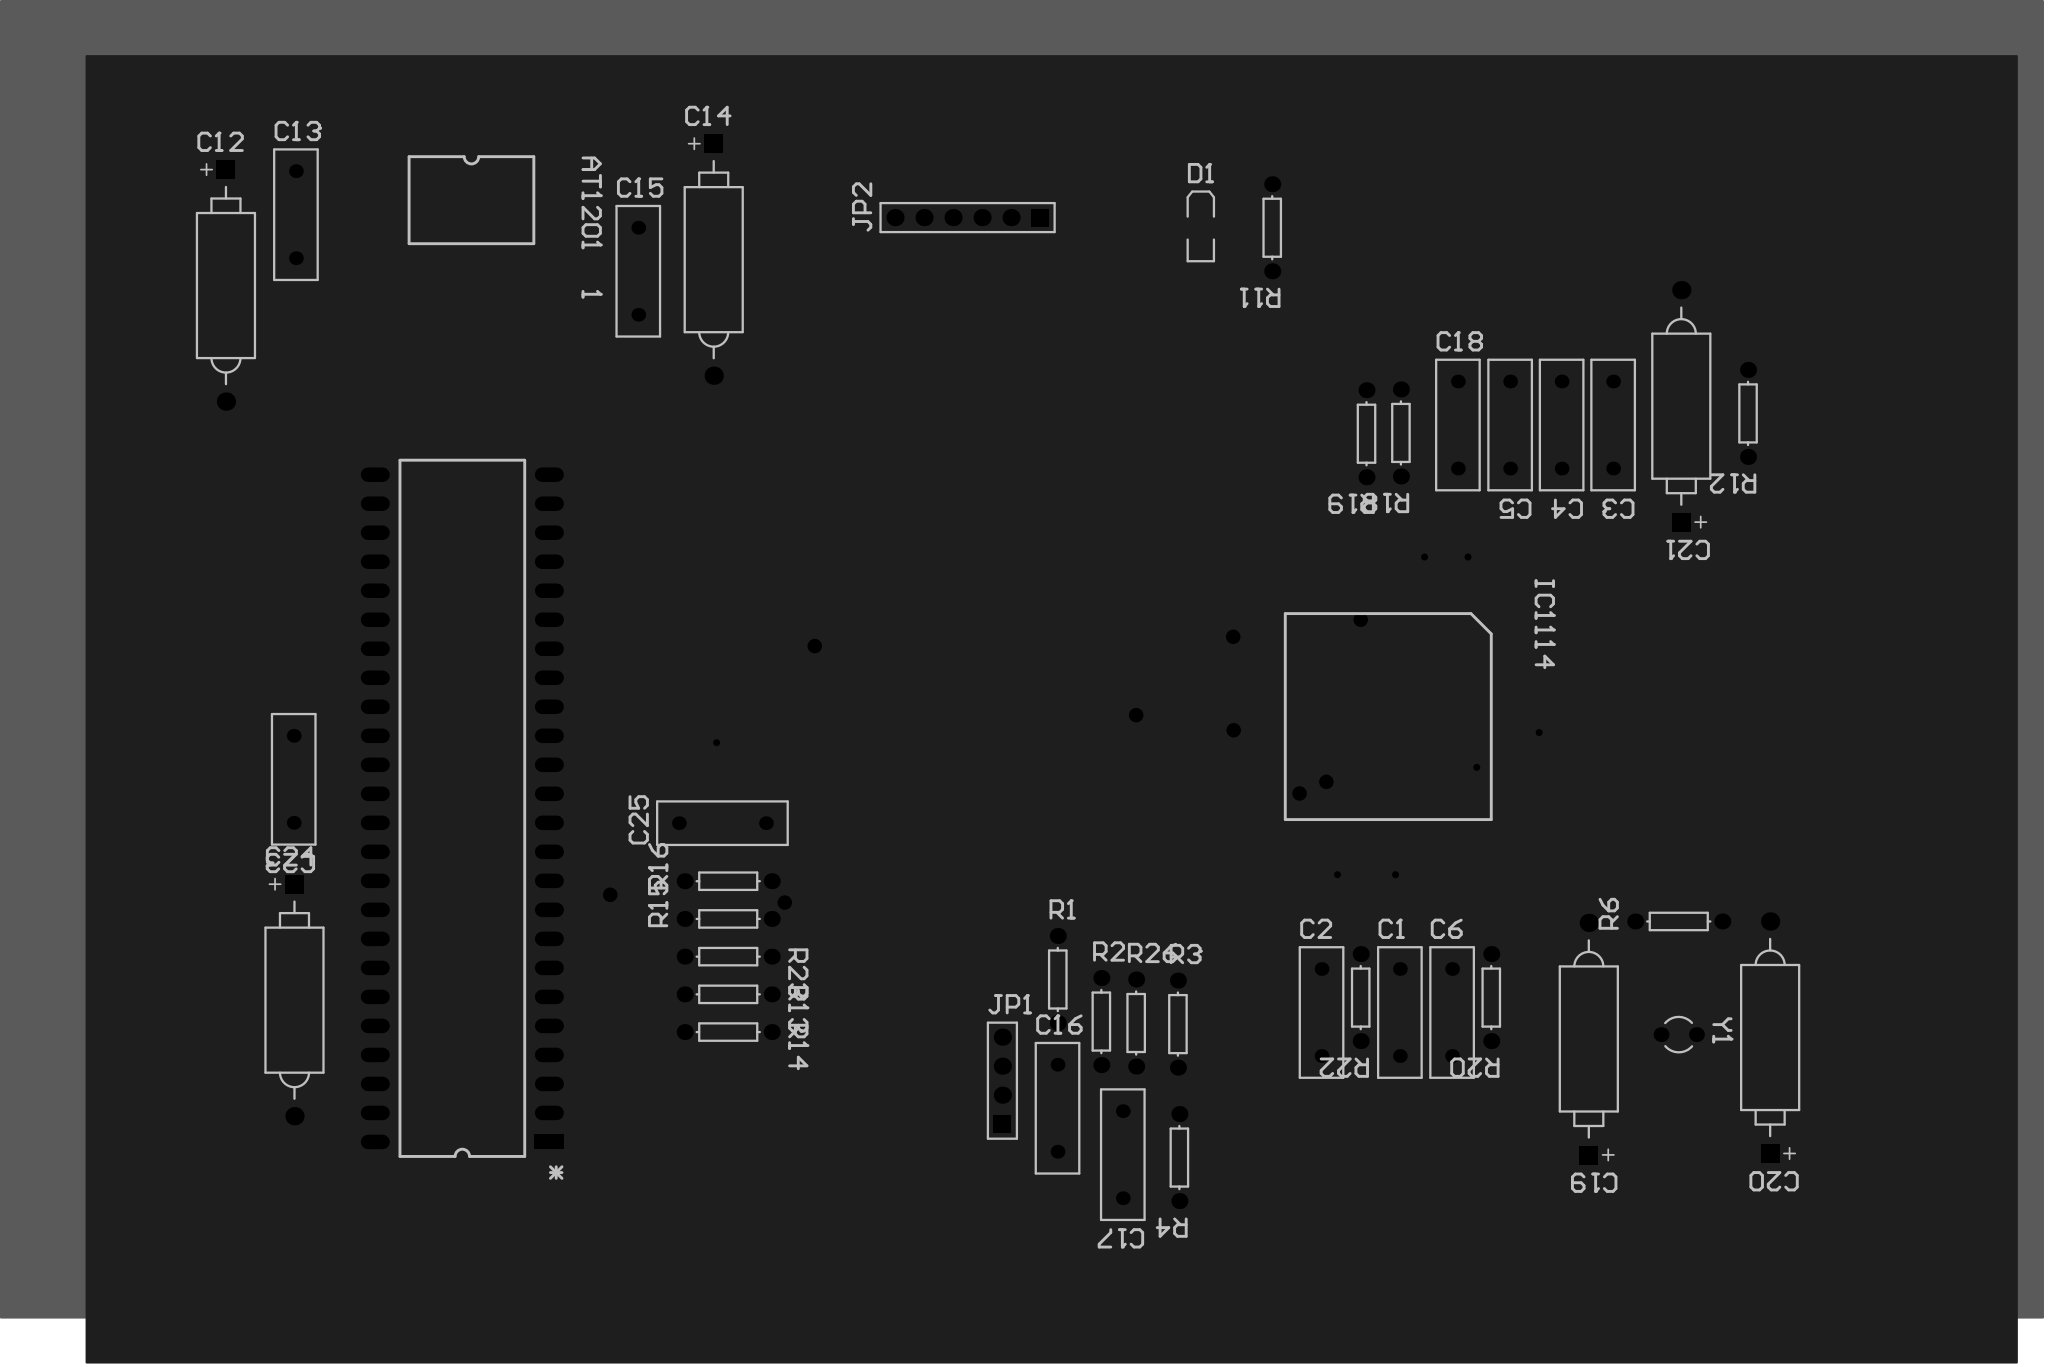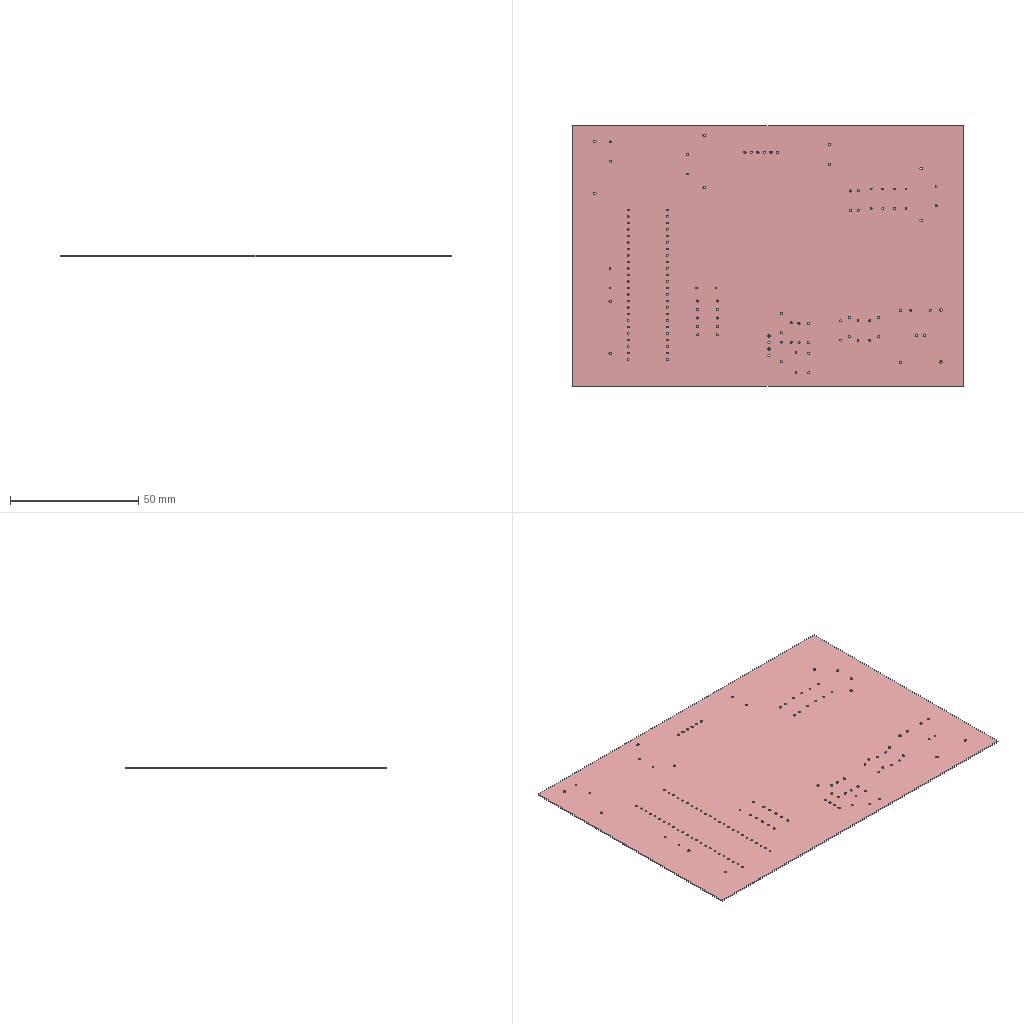Circuit board layout | Altium Designer | box 152.4 x 101.6 x 0.4 mm
Layer stack:
# Altium Designer layer stack of  (unit mm; dielectric type: 0 none, 1 core, 2 prepreg, 3 surface material)
index,name,kind,layer,copper_thickness_mm,dielectric_type,dielectric_thickness_mm,dielectric_material,dielectric_constant
0,Top Paste Mask Layer,other,,,,,,
1,Top Silkscreen Layer,other,,,,,,
2,Top Solder Mask Layer,dielectric,,,3,0.0102,Solder Resist,3.5
3,Top Layer,copper,Top Layer,0.0356,,,,
4,Dielectric 1,dielectric,,,3,0.32,FR-4,4.8
5,Bottom Layer,copper,Bottom Layer,0.0356,,,,
6,Bottom Solder Mask Layer,dielectric,,,3,0.0102,Solder Resist,3.5
7,Bottom Silkscreen Layer,other,,,,,,
8,Bottom Paste Mask Layer,other,,,,,,
# drill layer pairs: low layer,high layer
drill_pair,Top Layer,Bottom Layer
Part placement:
Designator,Comment,Layer,Footprint,Center-X(mm),Center-Y(mm),Rotation
Y1,,TopLayer,R38,223.17,104.998,270
R1,Res1,TopLayer,AXIAL-0.3,168.806,109.824,90
R26,,TopLayer,AXIAL-0.3,175.667,106.014,90
R23,,TopLayer,AXIAL-0.3,139.954,111.825,0
R22,,TopLayer,AXIAL-0.3,195.326,108.239,270
R20,,TopLayer,AXIAL-0.3,206.756,108.239,270
R19,,TopLayer,AXIAL-0.3,195.834,157.607,270
R18,,TopLayer,AXIAL-0.3,198.846,157.676,270
R16,,TopLayer,AXIAL-0.3,139.954,118.429,180
R15,,TopLayer,AXIAL-0.3,139.954,115.127,180
R14,,TopLayer,AXIAL-0.3,139.954,105.221,0
R13,,TopLayer,AXIAL-0.3,139.954,108.523,0
R12,,TopLayer,AXIAL-0.3,229.235,159.385,270
R11,,TopLayer,AXIAL-0.3,187.579,175.641,270
R6,,TopLayer,AXIAL-0.3,223.17,114.904,180
R4,,TopLayer,AXIAL-0.3,179.451,94.234,270
R3,,TopLayer,AXIAL-0.3,179.324,105.918,90
R2,,TopLayer,AXIAL-0.3,172.619,106.141,90
JP2,JUMPER6_1.27MM,TopLayer,HDR1X6,160.909,176.53,180
JP1,Header 4,TopLayer,HDR1X4,163.957,100.965,90
IC1114,Component_1,TopLayer,Quad48,197.739,132.842,270
D1,LED2,TopLayer,3.2X1.6X1.1,181.327,175.61,90
C25,,TopLayer,RAD-0.3,139.446,123.509,180
C24,,TopLayer,POLAR0.8,101.981,108.015,90
C23,,TopLayer,RAD-0.3,101.915,127.35,270
C21,,TopLayer,POLAR0.8,223.393,160.02,270
C20,,TopLayer,POLAR0.8,231.171,104.744,270
C19,,TopLayer,POLAR0.8,215.296,104.617,270
C18,,TopLayer,RAD-0.3,203.835,158.369,90
C16,,TopLayer,RAD-0.3,168.783,98.552,90
C15,,TopLayer,RAD-0.3,132.08,171.831,90
C14,,TopLayer,POLAR0.8,138.684,172.847,90
C13,,TopLayer,RAD-0.3,102.108,176.784,90
C12,,TopLayer,POLAR0.8,95.982,170.58,90
C6,,TopLayer,RAD-0.3,203.327,106.934,90
C5,,TopLayer,RAD-0.3,208.407,158.369,270
C4,,TopLayer,RAD-0.3,212.916,158.369,270
C3,,TopLayer,RAD-0.3,217.424,158.369,270
C2,,TopLayer,RAD-0.3,191.897,106.934,90
C1,,TopLayer,RAD-0.3,198.755,106.934,90
AT1201  1,AT1201_SOT25,TopLayer,SOP6,117.475,178.054,0
*,Component_2,TopLayer,DIP48,116.677,124.81,180
C17,,TopLayer,RAD-0.3,174.498,94.488,270
Pad and via stacks:
# Altium Designer via and pad stacks of  (unit mm). Each distinct definition once, with the count of objects using it.
# via: kind,start_layer,end_layer,hole_mm,diameter_mm,mode(0 simple;1 top-mid-bottom;2 full stack),diameter_per_layer,count,example_net
# pad: kind,layer,hole_mm,hole_type(0 round;1 square;2 slot),plating,top_size,top_shape(1 round;2 rect;3 octagon;9 rounded rect),mid_size,bottom_size,mode,footprint,size_per_layer,count,example
pad,Multi-Layer,0.7,0,plated,1.3x1.3,1,1.3x1.3,1.3x1.3,0,R38,,2,Y1.1
pad,Multi-Layer,0.85,0,plated,1.4x1.4,1,1.4x1.4,1.4x1.4,0,AXIAL-0.3,,34,R1.2
pad,Multi-Layer,0.9,0,plated,1.5x1.5,2,1.5x1.5,1.5x1.5,0,HDR1X6,,1,JP2.1
pad,Multi-Layer,0.9,0,plated,1.5x1.5,1,1.5x1.5,1.5x1.5,0,HDR1X6,,5,JP2.2
pad,Multi-Layer,0.9,0,plated,1.5x1.5,1,1.5x1.5,1.5x1.5,0,HDR1X4,,3,JP1.4
pad,Multi-Layer,0.9,0,plated,1.5x1.5,2,1.5x1.5,1.5x1.5,0,HDR1X4,,1,JP1.1
pad,Multi-Layer,0.7,0,plated,1.2x1.2,1,1.2x1.2,1.2x1.2,0,RAD-0.3,,26,C25.2
pad,Multi-Layer,1,0,plated,1.6x1.6,1,1.6x1.6,1.6x1.6,0,POLAR0.8,,6,C24.2
pad,Multi-Layer,1,0,plated,1.6x1.6,2,1.6x1.6,1.6x1.6,0,POLAR0.8,,6,C24.1
pad,Multi-Layer,0.635,0,plated,2.54x1.27,2,2.54x1.27,2.54x1.27,0,DIP48,,1,*.1
pad,Multi-Layer,0.635,0,plated,2.54x1.27,1,2.54x1.27,2.54x1.27,0,DIP48,,47,*.2
pad,Top Layer,0,0,plated,0.635x2.54,2,0.635x2.54,0.635x2.54,0,Quad48,,47,IC1114.48
pad,Top Layer,0,0,plated,0.635x2.54,1,0.635x2.54,0.635x2.54,0,Quad48,,1,IC1114.1
pad,Top Layer,0,0,plated,1.5x1.5,2,1.5x1.5,1.5x1.5,0,3.2X1.6X1.1,,2,D1.1
pad,Top Layer,0,0,plated,2.54x1.27,2,2.54x1.27,2.54x1.27,0,SOP6,,1,AT1201  1.1
pad,Top Layer,0,0,plated,2.54x1.27,1,2.54x1.27,2.54x1.27,0,SOP6,,4,AT1201  1.2
via,Top Layer,Bottom Layer,0.7112,1.27,0,,9,BDA
via,Top Layer,Bottom Layer,0.3048,0.61,0,,7,VCC
Copper pours:
name,layer,net,type(0 solid;1 hatched;2 none)
Top Layer-GND,Top Layer,GND,0
Bottom Layer-GND,Bottom Layer,GND,0
Design rules, without the lines most boards share:
# Altium Designer design rules of  (exported by Altium Designer, unit mm)
# columns: name | kind | enabled | priority | scope1 | scope2 | descriptor | typed fields (field=value)
ComponentClearance_1 | 24 | enabled | 1 | All | All | Component Clearance Constraint ( Horizontal Gap = 10mil, Vertical Gap = 10mil ) (All),(All)  | gap=0.254
Clearance | 0 | enabled | 1 | All | All | Clearance Constraint (Gap=10mil) (All),(All) | gap=0.254
Clearance_1 | 63 | enabled | 1 | All | All | Board Clearance Constraint (Gap=0mil) (All) |
ComponentClearance | 52 | enabled | 1 | All | All | Hole To Hole Clearance (Gap=10mil) (All),(All) | gap=0.254
Width | 2 | enabled | 1 | All | All | Width Constraint (Min=5mil) (Max=100mil) (Preferred=10mil) (All) |
DiffPairsRouting | 51 | enabled | 1 | All | All | Differential Pairs Uncoupled Length using the Gap Constraints (Min=10mil) (Max=10mil) (Prefered=10mil)  and Width Constraints (Min=15mil) (Max=15mil) (Prefered=15mil) (All) |
RoutingVias | 11 | enabled | 1 | All | All | Routing Via (MinHoleWidth=28mil) (MaxHoleWidth=28mil) (PreferredHoleWidth=28mil) (MinWidth=50mil) (MaxWidth=50mil) (PreferedWidth=50mil) (All) | via_min_hole=0.7112 via_max_hole=0.7112 via_preferred_diameter=1.27 via_preferred_hole=0.7112
PlaneConnect | 6 | enabled | 1 | All | All | Power Plane Connect Rule(Relief Connect )(Expansion=20mil) (Conductor Width=10mil) (Air Gap=10mil) (Entries=4) (All) | relief_conductor_width=0.254 relief_entries=4 relief_expansion=0.508
PolygonConnect | 20 | enabled | 1 | (InNet('GND')) | All | Polygon Connect Rule(Relief Connect )(Conductor Width=10mil) (Relief Angle=90 Angle) (Entries=4) (Air Gap Width=10mil) ((InNet('GND'))),(All) | connect_style(0=relief,1=direct,2=none)=0 relief_conductor_width=0.254 relief_entries=4
PasteMaskExpansion | 14 | enabled | 1 | All | All | Paste Mask Expansion (Expansion =0mil) (All) | expansion=0
SolderMaskExpansion | 13 | enabled | 1 | All | All | Solder Mask Expansion (Expansion =4mil) (All) | expansion=0.1016